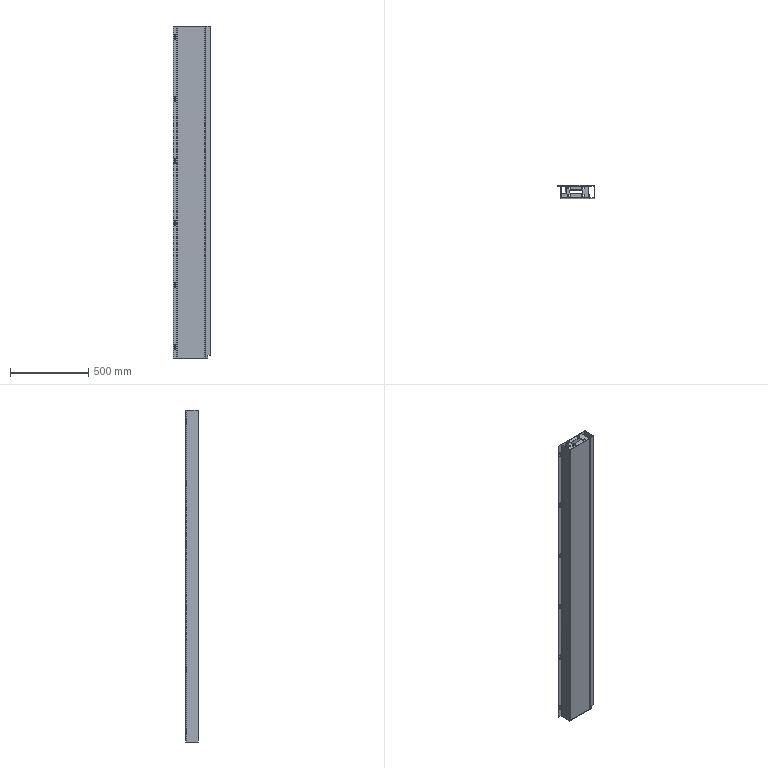Part | SolidWorks | features Fillet 6, ICE 5, Extrusion 1, MirrorSolid 1 | 5 solids | 154 faces | box 240 x 80 x 2116 mm | volume 3439932 mm3 | plane 88 | cylinder 66 | commonest cylinder face diameters 10 x24 9 x18 2 x9 6 x8 25 x6 8 x1